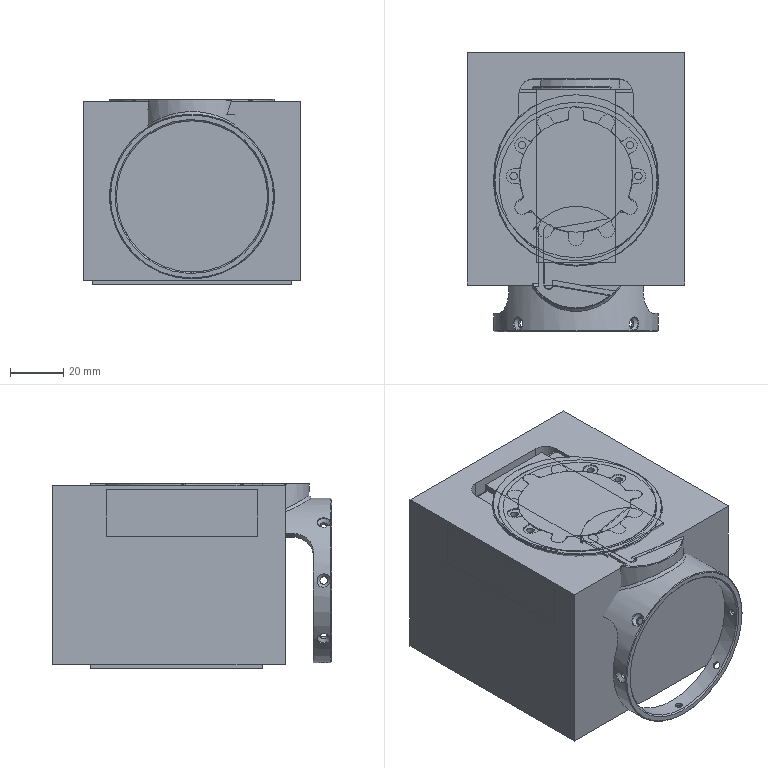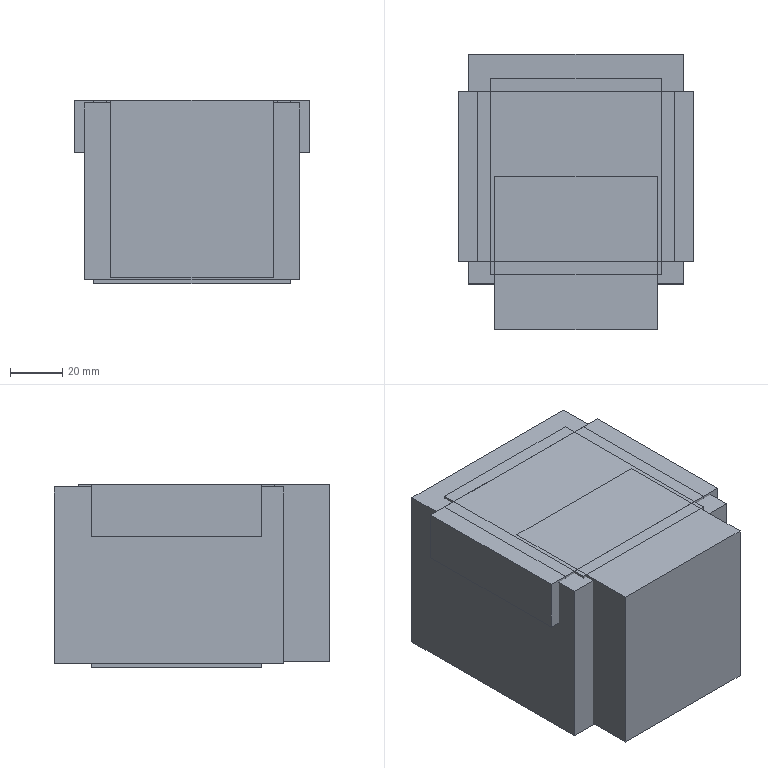CAM job | NX | 3-axis milling, 5-axis milling, drilling | part box 82 x 105.2 x 70 mm | stock box 90 x 105.2 x 70 mm
Tools:
number,name,description,diameter,corner_radius,flute_length,length,flutes
22,光刀D2,Milling Tool-5 Parameters,2.0,0.0,5.0,12.0,4
14,光刀D2.5,,2.5,0.0,7.0,13.0,4
7,光刀D4,Milling Tool-5 Parameters,4.0,0.0,10.0,15.0,4
6,光刀D6,Milling Tool-5 Parameters,6.0,0.0,15.0,16.0,4
8,光刀D8,,8.0,0.0,20.0,30.0,4
19,光刀D10,,10.0,0.0,25.0,35.0,4
7,粗刀D4,Milling Tool-5 Parameters,4.0,0.0,10.0,11.0,4
27,粗刀D6,Milling Tool-5 Parameters,6.0,0.0,15.0,18.0,4
28,粗刀D8,,8.0,0.0,22.0,35.0,2
15,粗刀D10,,10.0,0.0,25.0,40.0,2
18,粗刀D16,,16.0,0.0,40.0,68.1,2
11,倒角刀D4,Chamfer Mill,4.0,0.0,2.0,20.0,2
26,倒角刀D6,Chamfer Mill,6.0,0.0,3.0,62.433,2
29,倒角刀D5,Chamfer Mill,5.0,0.0,2.5,10.0,2
1,中心钻D6,Spot Drill,6.0,3.0,0.0,10.0,2
17,钻头D1.7,Drilling Tool,1.6,0.0,10.0,25.0,2
19,钻头D2.8,Drilling Tool,2.8,0.0,10.0,20.0,2
16,钻头D3.2,Drilling Tool,3.2,0.0,10.0,20.0,2
24,球刀D2R1,Milling Tool-Ball Mill,2.0,1.0,4.0,18.578,2
0,球刀D3R1.5,Milling Tool-Ball Mill,3.0,1.5,5.0,17.89,2
20,飞刀D50,,50.0,0.0,50.0,75.0,2
9,45度燕尾刀D6,Milling Tool-5 Parameters,6.0,0.0,1.5,1.5,2
0,45度燕尾刀D5,,5.0,0.0,1.25,1.25,4
0,45度燕尾刀D2,Milling Tool-5 Parameters,2.0,0.0,0.55,0.55,2
25,M2P0.4螺纹刀单齿柄4,   ,1.55,0.0,0.4,10.0,2
0,T型刀D20-8,Milling Tool-T Cutter,20.0,,8.0,70.0,4
21,鼓形刀D8R1.5,Milling Tool-Barrel,8.0,,3.0,32.0,4
10,D10加长刀,Milling Tool-5 Parameters,10.0,0.0,62.5,75.0,2
Operations:
program,operation,operation_type,tool,method,geometry_group,spindle_rpm,surface_speed,feed_per_tooth,feed_cut,feed_plunge,cut_length_mm,path_length_mm,cut_time_min,machine_time_min
A-1,单向轮廓精光,PlanarMilling,飞刀D50,光,WO-1,4000.0,628.318,0.25,2000.0,100.0,848.4,1577.6,0.4242,0.4971
A-1,单向轮廓精光_COPY,PlanarMilling,飞刀D50,光,WO-1,4000.0,628.318,0.125,1000.0,100.0,282.8,403.2,0.2828,0.2948
A-2,单向轮廓精光_1,PlanarMilling,光刀D10,光,WO-1,8000.0,251.327,0.0375,1200.0,100.0,174.8,254.8,0.1457,0.1537
A-3,倒角刀D6._1,PlanarMilling,倒角刀D6,FINISH,WO-1,7500.0,141.372,0.08,1200.0,100.0,158.4,224.8,0.132,0.1386
B-1,单向轮廓精光_2,PlanarMilling,飞刀D50,光,WO-2,5500.0,863.938,0.0727,800.0,100.0,344.918,418.918,0.4311,0.4385
B-2,外形动态铣,SurfaceContour,粗刀D16,ROUGHING,WO-2,8500.0,267.035,0.2647,4500.0,100.0,3338.892,3794.36,0.6634,0.7319
B-2,轮廓开粗,PlanarMilling,粗刀D16,ROUGHING,WO-2,5000.0,251.327,0.25,2500.0,100.0,232.8,516.49,0.0582,0.0866
B-13,单向轮廓精光_2_COPY,PlanarMilling,飞刀D50,光,WO-2,5500.0,863.938,0.0727,800.0,100.0,126.119,200.119,0.1576,0.165
B-3,外形动态铣_COPY,SurfaceContour,粗刀D10,ROUGHING,WO-2,8500.0,267.035,0.2059,3500.0,100.0,6465.325,17034.288,1.715,3.613
B-3,区域轮廓铣,SurfaceContour,粗刀D10,光,WO-2,7000.0,219.911,0.2857,4000.0,100.0,13934.689,14303.932,3.484,3.521
B-3,轮廓开粗_1,PlanarMilling,粗刀D10,ROUGHING,WO-2,7500.0,235.619,0.2667,4000.0,100.0,36.333,146.493,0.0091,0.0201
B-4,中心钻,HoleDrilling,倒角刀D4,DRILL,WO-2,2600.0,49.009,0.0385,200.0,100.0,18.0,607.051,0.09,0.1489
B-4,中心钻_COPY,HoleDrilling,倒角刀D4,DRILL,WO-2,2600.0,49.009,0.0385,200.0,100.0,7.2,292.926,0.036,0.0646
B-4,中心钻_COPY_COPY,HoleDrilling,倒角刀D4,DRILL,WO-2,2600.0,49.009,0.0385,200.0,100.0,25.2,876.857,0.126,0.2112
B-5,高版本钻孔,HoleDrilling,钻头D1.7,DRILL,WO-2,4000.0,20.106,0.0187,150.0,0.0,34.952,259.19,0.0466,0.069
B-5,高版本钻孔_COPY,HoleDrilling,钻头D1.7,DRILL,WO-2,4000.0,20.106,0.0187,150.0,0.0,33.084,181.93,0.0424,0.0573
B-6,高版本钻孔_COPY_COPY,HoleDrilling,钻头D3.2,DRILL,WO-2,4000.0,40.212,0.0125,100.0,0.0,53.952,279.635,0.1098,0.1324
B-7,高版本钻孔_COPY_COPY_COPY,HoleDrilling,钻头D2.8,DRILL,WO-2,3000.0,26.389,0.0167,100.0,0.0,140.165,790.592,0.3039,0.3689
B-8,高版本钻孔_COPY_COPY_COPY_COPY,HoleDrilling,倒角刀D5,DRILL,WO-2,1200.0,18.85,0.0167,40.0,0.0,70.0,720.427,0.4375,0.5025
B-10,单向轮廓精光_3,PlanarMilling,光刀D6,光,WO-2,8000.0,150.796,0.0219,700.0,100.0,108.193,351.235,0.1546,0.1789
B-10,单向轮廓精光_3_COPY,PlanarMilling,光刀D6,光,WO-2,8000.0,150.796,0.0219,700.0,100.0,82.239,322.239,0.1175,0.1415
B-10,单向轮廓精光_3_COPY_1,PlanarMilling,光刀D6,光,WO-2,8000.0,150.796,0.0219,700.0,100.0,283.9,539.601,0.4056,0.4311
B-10,单向轮廓精光_3_COPY_1_COPY_COPY_COPY_COPY_COPY,PlanarMilling,光刀D6,光,WO-2,7000.0,131.947,0.0429,1200.0,100.0,81.397,172.837,0.0678,0.077
B-11,单向轮廓精光_3_COPY_1_COPY,PlanarMilling,光刀D2.5,光,WO-2,12000.0,94.248,0.0312,1500.0,100.0,1074.852,1579.274,0.7166,0.767
B-11,单向轮廓精光_3_COPY_1_COPY_COPY,PlanarMilling,光刀D2.5,光,WO-2,12000.0,94.248,0.0146,700.0,100.0,138.88,334.713,0.1984,0.218
B-12,单向轮廓精光_3_COPY_1_COPY_COPY_COPY_COPY,PlanarMilling,光刀D4,光,WO-2,12000.0,94.248,0.0146,700.0,100.0,162.752,384.661,0.2325,0.2547
B-12,单向轮廓精光_3_COPY_1_COPY_COPY_COPY,PlanarMilling,光刀D4,光,WO-2,12000.0,94.248,0.0146,700.0,100.0,175.874,348.529,0.2512,0.2685
B-12,底壁铣选底,VolumeBased25DMillingOperation,光刀D4,FINISH,WO-2,8000.0,201.062,0.0375,1200.0,100.0,272.617,369.317,0.2272,0.2369
B-14,单向轮廓精光_4,PlanarMilling,D10加长刀,光,WO-2,4500.0,141.372,0.0778,700.0,100.0,873.424,1795.444,1.248,1.34
B-15,单向轮廓精光_5,PlanarMilling,光刀D8,光,WO-2,8000.0,251.327,0.0375,1200.0,100.0,82.68,184.08,0.0689,0.079
B1602,VARIABLE_CONTOUR_COPY_2,SurfaceContour,45度燕尾刀D6,光,MCS-2,8000.0,150.796,0.1875,3000.0,100.0,1178.784,1205.143,0.3929,0.3956
B1602,VARIABLE_CONTOUR_COPY_2_COPY,SurfaceContour,45度燕尾刀D6,光,MCS-2,8000.0,150.796,0.1875,3000.0,100.0,1178.784,1205.143,0.3929,0.3956
B1605,VARIABLE_AXIS_GUIDING_CURVES_COPY,SurfaceContour,球刀D2R1,METHOD,WO-2,12000.0,113.097,0.125,3000.0,100.0,11955.822,12022.13,3.985,3.992
B1605,VARIABLE_AXIS_GUIDING_CURVES_COPY_1,SurfaceContour,球刀D2R1,METHOD,MCS-2,12000.0,113.097,0.125,3000.0,100.0,234.218,316.974,0.0781,0.0863
B1605_COPY,VARIABLE_AXIS_GUIDING_CURVES_COPY_2_COPY,SurfaceContour,球刀D3R1.5,METHOD,MCS-2,16000.0,150.796,0.0781,2500.0,100.0,13431.952,13943.358,5.373,5.424
B1604,VARIABLE_CONTOUR_COPY_2_COPY_1,SurfaceContour,45度燕尾刀D6,光,MCS-2,12000.0,226.195,0.125,3000.0,100.0,2340.368,2366.699,0.7801,0.7828
B1604,VARIABLE_CONTOUR_COPY_2_COPY_1_COPY,SurfaceContour,45度燕尾刀D6,光,MCS-2,12000.0,226.195,0.125,3000.0,100.0,2787.114,2813.445,0.929,0.9317
B-9,外形动态铣_COPY_1,SurfaceContour,粗刀D16,ROUGHING,WO-2,8500.0,267.035,0.2647,4500.0,100.0,5209.395,5946.006,1.153,1.263
B1601,VARIABLE_CONTOUR_COPY_1,SurfaceContour,鼓形刀D8R1.5,光,MCS-2,8000.0,201.062,0.0625,2000.0,100.0,361.226,406.598,0.1806,0.1852
B1601,VARIABLE_CONTOUR_COPY_1_COPY,SurfaceContour,鼓形刀D8R1.5,光,MCS-2,8000.0,201.062,0.0625,2000.0,100.0,968.506,1012.99,0.4843,0.4887
B1606,倒角刀D6._COPY_COPY_COPY_1,PlanarMilling,倒角刀D4,FINISH,WO-2,7500.0,141.372,0.08,1200.0,100.0,26.457,102.457,0.022,0.0296
B1606,倒角刀D6.,PlanarMilling,倒角刀D4,FINISH,WO-2,7500.0,141.372,0.08,1200.0,100.0,90.33,262.899,0.0753,0.0925
B1606,倒角刀D6._COPY,PlanarMilling,倒角刀D4,FINISH,WO-2,7500.0,141.372,0.08,1200.0,100.0,57.488,145.288,0.0479,0.0567
B1606,倒角刀D6._COPY_COPY,PlanarMilling,倒角刀D4,FINISH,WO-2,7500.0,141.372,0.08,1200.0,100.0,38.492,126.891,0.0321,0.0409
B1606,倒角刀D6._COPY_COPY_COPY,PlanarMilling,倒角刀D4,FINISH,WO-2,7500.0,141.372,0.08,1200.0,100.0,69.561,239.043,0.058,0.0749
B1606,倒角刀D6._COPY_COPY_COPY_2,PlanarMilling,倒角刀D4,FINISH,WO-2,7500.0,94.248,0.0267,400.0,100.0,39.25,382.05,0.0981,0.1324
B1606,中心钻_1,HoleDrilling,倒角刀D4,DRILL,WO-2,2600.0,49.009,0.0385,200.0,100.0,8.4,245.4,0.042,0.0657
B1606,中心钻_1_COPY,HoleDrilling,倒角刀D4,DRILL,WO-2,2600.0,49.009,0.0385,200.0,100.0,8.4,294.126,0.042,0.0706
B1606,倒角刀D6._COPY_COPY_COPY_2_COPY,PlanarMilling,倒角刀D4,FINISH,WO-2,7500.0,94.248,0.0267,400.0,100.0,389.164,600.664,0.9729,0.9941
B1606,点线倒角,SurfaceContour,倒角刀D4,METHOD,MCS-2,5000.0,94.248,0.08,800.0,100.0,124.791,783.856,0.156,0.2219
B1615_COPY,倒角刀D6._COPY_COPY_COPY_2_COPY_COPY,PlanarMilling,倒角刀D6,FINISH,WO-2,5500.0,103.673,0.0364,400.0,100.0,163.495,348.095,0.4087,0.4272
B1615_COPY,倒角刀D6._COPY_COPY_COPY_2_COPY_COPY_COPY,PlanarMilling,倒角刀D6,FINISH,WO-2,5500.0,103.673,0.0364,400.0,100.0,164.123,348.523,0.4103,0.4287
B1607,M3螺纹铣,ThreadMilling,M2P0.4螺纹刀单齿柄4,光,WO-2,7000.0,34.086,0.0214,300.0,100.0,56.397,309.324,0.188,0.2133
B1607,M3螺纹铣_COPY,ThreadMilling,M2P0.4螺纹刀单齿柄4,光,WO-2,7000.0,34.086,0.0214,300.0,100.0,60.688,363.586,0.2023,0.2326
B1612,多轴去毛刺,TpMultiAxisDeburring,倒角刀D4,METHOD,MCS-2,5000.0,94.248,0.04,400.0,200.0,338.235,377.606,0.8534,0.8534
B1610,VARIABLE_CONTOUR_COPY_1_COPY_1,SurfaceContour,粗刀D6,光,MCS-2,7000.0,131.947,0.125,3500.0,100.0,2665.847,3019.886,0.7617,0.7971
B1611,CONTOUR_PROFILE_COPY,SurfaceContour,光刀D4,METHOD,MCS-2,4500.0,56.549,0.0444,800.0,200.0,626.583,660.406,0.8409,0.8443
B1613,VARIABLE_CONTOUR_COPY_2_COPY_2,SurfaceContour,45度燕尾刀D2,光,MCS-2,8000.0,50.266,0.0125,200.0,100.0,7.764,60.186,0.0388,0.0441
B1613,VARIABLE_CONTOUR_COPY_2_COPY_2_INSTANCE,SurfaceContour,45度燕尾刀D2,光,MCS-2,8000.0,50.266,0.0125,200.0,100.0,7.764,60.186,0.0388,0.0441
B1613,VARIABLE_CONTOUR_COPY_2_COPY_2_INSTANCE_1,SurfaceContour,45度燕尾刀D2,光,MCS-2,8000.0,50.266,0.0125,200.0,100.0,7.764,60.186,0.0388,0.0441
B1613_COPY,VARIABLE_CONTOUR_COPY_2_COPY_2_COPY,SurfaceContour,45度燕尾刀D6,光,MCS-2,2800.0,52.779,0.0714,400.0,100.0,309.955,354.022,0.7749,0.7793
B1614,可变轮廓铣,SurfaceContour,粗刀D8,METHOD,MCS-2,7000.0,175.929,0.1786,2500.0,100.0,5159.229,5237.856,2.064,2.072
C-1,外形动态铣_1,SurfaceContour,粗刀D16,ROUGHING,WO-3,5500.0,276.46,0.3182,3500.0,100.0,10288.728,10613.898,2.919,2.972
C-2,单向轮廓精光_6,PlanarMilling,T型刀D20-8,光,WO-3,1500.0,94.248,0.1333,800.0,100.0,2055.613,2746.58,2.57,2.639
C-3,踩R角,Operation,光刀D10,DRILL,WO-3,2000.0,62.0,0.05,400.0,0.0,117.0,289.016,0.2925,0.3097
C-3,底壁铣选底_1,VolumeBased25DMillingOperation,光刀D10,FINISH,WO-3,8000.0,201.062,0.0375,1200.0,100.0,541.992,677.292,0.4517,0.4652
C-3,单向轮廓精光_7,PlanarMilling,光刀D10,光,WO-3,8000.0,251.327,0.0375,1200.0,100.0,1157.043,1439.919,0.9642,0.9925
D-1,轮廓开粗_2,PlanarMilling,粗刀D10,ROUGHING,WO-4,7000.0,219.911,0.1786,2500.0,100.0,735.165,751.025,0.2941,0.2957
D-1,轮廓开粗_2_COPY,PlanarMilling,粗刀D10,ROUGHING,WO-4,5500.0,172.788,0.1364,1500.0,100.0,113.837,136.837,0.0759,0.0782
D-2,中心孔,Operation,中心钻D6,DRILL,WO-4,2000.0,50.0,0.045,180.0,0.0,22.5,193.276,0.125,0.1421
D-3,钻头D2.9-,Operation,钻头D2.8,DRILL,WO-4,2500.0,22.0,0.04,200.0,0.0,57.071,273.733,0.2854,0.307
D-4,轮廓开粗_3,PlanarMilling,粗刀D4,ROUGHING,WO-4,8500.0,106.814,0.0588,2000.0,100.0,765.383,1294.571,0.3827,0.4356
D-4,轮廓开粗_3_COPY,PlanarMilling,粗刀D4,ROUGHING,WO-4,8500.0,106.814,0.0588,2000.0,100.0,418.652,441.344,0.2093,0.2116
D-5,单向轮廓精光_8,PlanarMilling,光刀D10,光,WO-4,8000.0,251.327,0.0375,1200.0,100.0,116.219,140.219,0.0968,0.0992
D-5,单向轮廓精光_8_COPY,PlanarMilling,光刀D10,光,WO-4,7000.0,219.911,0.0429,1200.0,100.0,381.27,395.27,0.3177,0.3191
D-6,单向轮廓精光_9,PlanarMilling,光刀D4,光,WO-4,8000.0,251.327,0.0375,1200.0,100.0,429.535,800.216,0.3579,0.395
D-6,单向轮廓精光_9_COPY,PlanarMilling,光刀D4,光,WO-4,8000.0,251.327,0.0375,1200.0,100.0,302.077,326.077,0.2517,0.2541
D-7,倒角刀D6._2,PlanarMilling,倒角刀D4,FINISH,WO-4,7500.0,141.372,0.08,1200.0,100.0,226.725,241.625,0.1889,0.1904
D-7,倒角刀D6._2_COPY,PlanarMilling,倒角刀D4,FINISH,WO-4,7500.0,94.248,0.0467,700.0,100.0,106.439,379.426,0.1521,0.1794
D-7,倒角刀D6._2_COPY_COPY,PlanarMilling,倒角刀D4,FINISH,WO-4,7500.0,94.248,0.0467,700.0,100.0,207,223,0.2957,0.2973
D-7,3轴去毛刺D6,TpMultiAxisDeburring,倒角刀D4,光,WO-4,8000.0,150.796,0.0625,1000.0,90.0,65.191,225.018,0.0674,0.0674
D-8,45度燕尾刀D5-C0.3,PlanarMilling,45度燕尾刀D5,ROUGHING,WO-4,7500.0,117.81,0.0667,2000.0,100.0,156.597,176.597,0.0783,0.0803
E-1,外形动态铣_2,SurfaceContour,粗刀D10,ROUGHING,WO-5,8500.0,267.035,0.2647,4500.0,100.0,4805.802,4828.642,1.058,1.062
E-1,轮廓开粗_4,PlanarMilling,粗刀D10,ROUGHING,WO-5,7500.0,235.619,0.2667,4000.0,100.0,2016.073,2082.457,0.504,0.5107
E-2,轮廓清角-D12,PlanarMilling,光刀D2,SEMI-FINISHING,WO-5,8500.0,53.407,0.0294,1000.0,100.0,990.034,1947.012,0.99,1.086
E-3,底壁铣选底_2,VolumeBased25DMillingOperation,光刀D10,FINISH,WO-5,8000.0,201.062,0.0375,1200.0,100.0,1651.92,2175.13,1.377,1.429
E-3,单向轮廓精光_10,PlanarMilling,光刀D10,光,WO-5,8000.0,251.327,0.0375,1200.0,100.0,649.555,704.555,0.5413,0.5468
E-4,3轴去毛刺D6_1,TpMultiAxisDeburring,倒角刀D6,光,WO-5,8000.0,150.796,0.0625,1000.0,90.0,467.748,502.689,0.4685,0.4685
E-5,单向轮廓精光_11,PlanarMilling,光刀D2,光,WO-5,8000.0,50.266,0.025,800.0,100.0,336.799,355.799,0.2807,0.2826
F-1,VARIABLE_CONTOUR_COPY_2_COPY_1_COPY_1,SurfaceContour,45度燕尾刀D6,光,MCS-6,12000.0,226.195,0.125,3000.0,100.0,2403.774,2430.194,0.8013,0.8039
F-1,VARIABLE_CONTOUR_COPY_2_COPY_1_COPY_1_COPY,SurfaceContour,45度燕尾刀D6,光,MCS-6,12000.0,226.195,0.125,3000.0,100.0,2403.592,2430.012,0.8012,0.8038
B1609,单向轮廓精光_4_COPY,PlanarMilling,D10加长刀,光,WO-2,6500.0,204.203,0.0269,700.0,100.0,489.413,671.413,0.6992,0.7174
B1609,单向轮廓精光_4_COPY_COPY,PlanarMilling,D10加长刀,光,WO-2,6500.0,204.203,0.0269,700.0,100.0,442.321,628.321,0.6319,0.6505